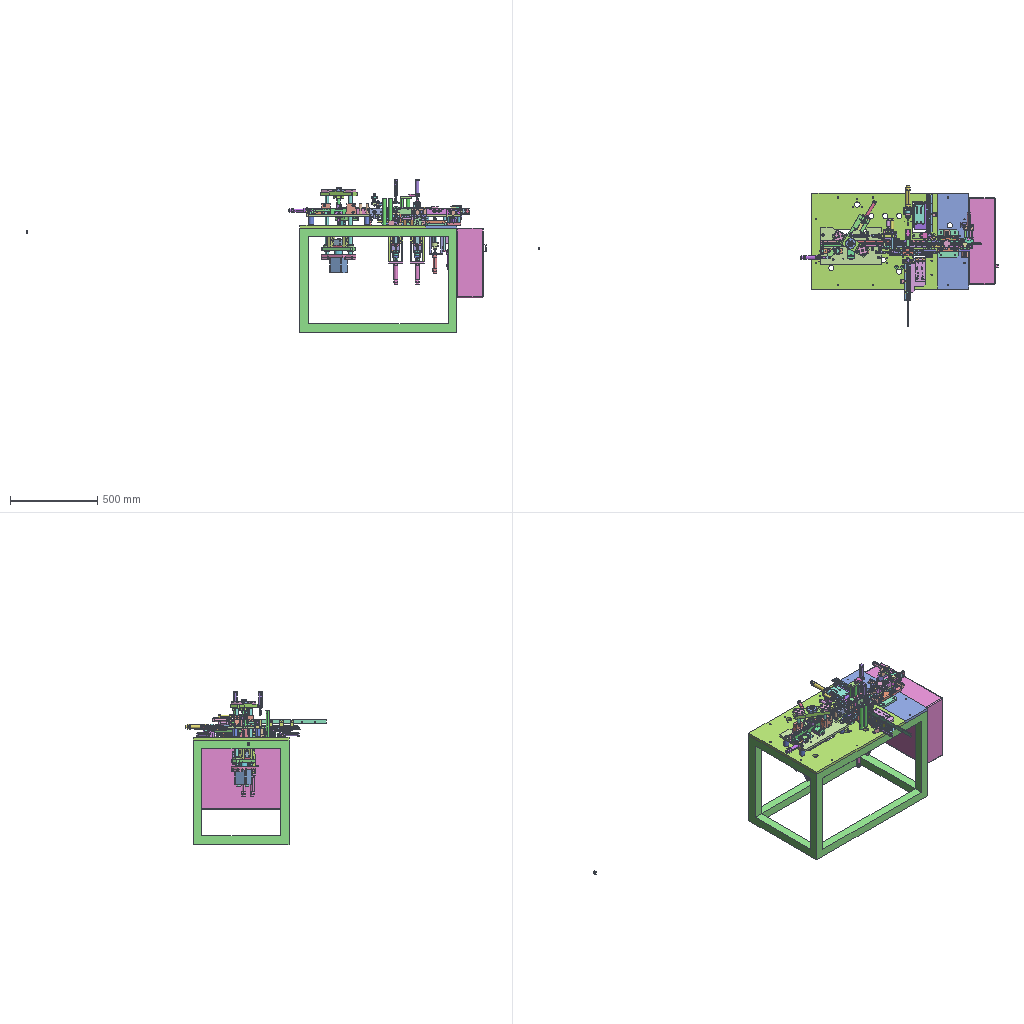Assembly | STEP file | 213 different items | 337 placed | box 2638 x 807 x 880 mm
Parts list (item | name | quantity | parent item | size | volume):
1 | magnet | x2 | in 180 magnet feeder main assembly | 5.5 x 14 x 19.5 mm | 770.904 mm3
2 | base plate | x1 | in 180 magnet feeder main assembly | 900 x 550 x 16 mm | 6619643 mm3
3 | vibratory feeder base plate | x2 | in vibratory feeder assembly | 116.996 x 12 x 60 mm | 79045 mm3
4 | vibratory feeder upper plate | x2 | in vibratory feeder assembly | 116.996 x 12 x 60 mm | 77221 mm3
5 | vibratory feeder support plate | x4 | in vibratory feeder assembly | 65 x 1 x 55 mm | 2512 mm3
6 | vibratory feeder support plate | x2 | in vibratory feeder assembly | 110 x 150 x 8 mm | 126115 mm3
7 | frame | x1 | in 180 magnet feeder main assembly | 550 x 600 x 900 mm | 18125000 mm3
8 | shell block | x3 | in 180 magnet feeder main assembly, 180 cup machine | 307.5 x 15.4 x 34 mm | 6550 mm3
9 | support plate 11 | x4 | in magnet input slingshot assembly | 8 x 160 x 68 mm | 53075 mm3
10 | slingshot push rod cylinder seat | x2 | in magnet input slingshot assembly | 81 x 35 x 8 mm | 19658 mm3
11 | CDM2B20-50-XC8 | x2 | in magnet input slingshot assembly | 24 x 24 x 166 mm | 54436 mm3
12 | magnetic tile top shaft cylinder seat 2 | x2 | in magnet input slingshot assembly | 45 x 49 x 12 mm | 14964 mm3
13 | top shaft cylinder seat support plate 2 | x2 | in magnet input slingshot assembly | 45 x 65 x 16 mm | 36671 mm3
14 | magnetic tile top shaft slide seat | x2 | in magnet input slingshot assembly | 95 x 90 x 26 mm | 105605 mm3
15 | union seat 11 | x2 | in magnet input slingshot assembly | 40 x 20 x 11 mm | 4585 mm3
16 | magnetic tile top shaft slider | x2 | in magnet input slingshot assembly | 40 x 51 x 45 mm | 61253 mm3
17 | slide seat cover plate 4 | x4 | in magnet input slingshot assembly | 17 x 90 x 10 mm | 13210 mm3
18 | union | x2 | in magnet input slingshot assembly | 16 x 17 x 16 mm | 2228 mm3
19 | magnetic tile top shaft | x2 | in magnet input slingshot assembly | 19 x 14 x 158 mm | 23396 mm3
20 | top shaft | x2 | in magnet input slingshot assembly | 8 x 11.5 x 178 mm | 13034 mm3
21 | union 1 | x2 | in magnet input slingshot assembly | 34 x 30 x 15 mm | 9782 mm3
22 | M6 screw | x2 | in magnet input slingshot assembly | 21 x 11 x 11 mm | 825.269 mm3
23 | CDM2B20-75 | x2 | in magnet input slingshot assembly | 24 x 24 x 166 mm | 54436 mm3
24 | push rod union | x2 | in magnet input slingshot assembly | 22 x 25 x 25 mm | 8188 mm3
25 | guide pin seat | x1 | in push slingshot assembly | 65 x 71 x 15 mm | 41839 mm3
26 | CDJ2B16_45_B_0_ | x5 | in push slingshot assembly, secondary slingshot input assembly, push material assembly | 18 x 22.7 x 120 mm | 25727 mm3
27 | slingshot displacement cylinder seat post | x4 | in push slingshot assembly, secondary slingshot input assembly | 20 x 20 x 155 mm | 47945 mm3
28 | push slingshot cylinder seat 2 | x2 | in push slingshot assembly, secondary slingshot input assembly | 60 x 26 x 20 mm | 12397 mm3
29 | slingshot track | x2 | in push slingshot assembly, secondary slingshot input assembly | 34 x 23.53 x 224 mm | 76613 mm3
30 | slingshot track fixed block | x3 | in push slingshot assembly | 11 x 40 x 22 mm | 2404 mm3
31 | secondary slingshot input track spacer block | x1 | in push slingshot assembly | 180 x 112 x 15 mm | 210119 mm3
32 | slingshot press plate | x1 | in push slingshot assembly | 375 x 20 x 5 mm | 36809 mm3
33 | pin seat 2 | x2 | in push slingshot assembly 9 | 35 x 30 x 8 mm | 7349 mm3
34 | pin seat 1 | x2 | in push slingshot assembly 9 | 35 x 30 x 8 mm | 7351 mm3
35 | slingshot push rod | x2 | in push slingshot assembly 9 | 16.072 x 21.6 x 67.5 mm | 5779 mm3
36 | union 4 | x2 | in push slingshot assembly, secondary slingshot input assembly | 12 x 21 x 12 mm | 1814 mm3
37 | lifting link plate | x2 | in push slingshot assembly, secondary slingshot input assembly | 13 x 40 x 8.5 mm | 2401 mm3
38 | fiber optic seat 2 | x2 | in push slingshot assembly, secondary slingshot input assembly | 13 x 13 x 13 mm | 515.025 mm3
39 | 16 union cap | x2 | in push slingshot assembly, secondary slingshot input assembly | 16 x 18 x 16 mm | 2782 mm3
40 | 16 union | x2 | in push slingshot assembly, secondary slingshot input assembly | 16 x 16 x 30 mm | 1888 mm3
41 | detection slide rod | x1 | in detection assembly | 60 x 12.5 x 13 mm | 5988 mm3
42 | detection union | x1 | in detection assembly | 19 x 12 x 14 mm | 1541 mm3
43 | slide seat | x2 | in detection assembly | 26 x 38 x 10 mm | 4433 mm3
44 | detection pin | x1 | in detection assembly | 6 x 6 x 30 mm | 164.036 mm3
45 | switch seat | x1 | in detection assembly | 35 x 29 x 12 mm | 1653 mm3
46 | detection post | x2 | in detection assembly | 16 x 16 x 60 mm | 11399 mm3
47 | push magnet block | x2 | in magnet input tile assembly | 25 x 14 x 20 mm | 5584 mm3
48 | push magnet union | x2 | in magnet input tile assembly | 10 x 10 x 18 mm | 1240 mm3
49 | push magnet block pin | x2 | in magnet input tile assembly | 3 x 3 x 14 mm | 98.96 mm3
50 | push magnet slide seat | x2 | in magnet input tile assembly | 34 x 28 x 32 mm | 18978 mm3
51 | push magnet slide seat spacer block | x2 | in magnet input tile assembly | 34 x 75 x 10 mm | 22964 mm3
52 | push magnet cylinder seat | x2 | in magnet input tile assembly | 34 x 25 x 28 mm | 8909 mm3
53 | push magnet seat spacer block 1 | x2 | in magnet input tile assembly | 34 x 20 x 17 mm | 10432 mm3
54 | magnet input block | x1 | in magnet input tile assembly | 60 x 40 x 64 mm | 101376 mm3
55 | CDJ2B10_30_C76_0_ | x2 | in magnet input tile assembly | 12.2 x 35.4 x 104 mm | 14245 mm3
56 | secondary slingshot input support plate | x1 | in secondary slingshot input assembly | 30 x 12 x 65 mm | 21465 mm3
57 | slingshot displacement cylinder seat | x1 | in secondary slingshot input assembly | 30 x 60 x 10 mm | 13257 mm3
58 | slider | x1 | in secondary slingshot input assembly | 80 x 40 x 8.5 mm | 14605 mm3
59 | slide seat 2 | x1 | in secondary slingshot input assembly | 65 x 30 x 80 mm | 57005 mm3
60 | secondary slingshot input track spacer block 1 | x1 | in secondary slingshot input assembly | 150 x 100 x 15 mm | 181436 mm3
61 | secondary slingshot input seat | x1 | in track assembly | 52 x 40 x 50 mm | 79247 mm3
62 | track spacer block 1 | x1 | in track assembly | 60 x 50 x 15 mm | 33797 mm3
63 | track spacer block 2 | x1 | in track assembly | 60 x 50 x 15 mm | 33477 mm3
64 | magnetizing track | x1 | in track assembly | 40 x 14 x 120 mm | 55579 mm3
65 | magnetizing side block 2 | x1 | in track assembly | 120 x 12.3 x 34.5 mm | 45166 mm3
66 | magnetizing side block | x1 | in track assembly | 120 x 12.3 x 34.5 mm | 44752 mm3
67 | secondary slingshot input side block 1 | x1 | in track assembly | 82.5 x 12.3 x 34.5 mm | 28839 mm3
68 | secondary slingshot input track | x1 | in track assembly | 40 x 14 x 82.5 mm | 35227 mm3
69 | iron shell displacement union | x1 | in track assembly | 15 x 22 x 39 mm | 5236 mm3
70 | iron shell displacement union seat | x1 | in track assembly | 27 x 25 x 18 mm | 8727 mm3
71 | track support post | x2 | in track assembly | 15 x 15 x 24 mm | 3445 mm3
72 | CDM2B20-50 | x1 | in track assembly | 24 x 24 x 166 mm | 54436 mm3
73 | insert limit | x8 | in track assembly, 180 magnet feeder main assembly | 20 x 12 x 10 mm | 1551 mm3
74 | iron shell positioning insert | x8 | in track assembly, 180 magnet feeder main assembly | 24 x 16.5 x 5 mm | 1571 mm3
75 | side block 5 | x1 | in track assembly | 12.1 x 101.5 x 34.5 mm | 29782 mm3
76 | side block 4 | x1 | in track assembly | 12.1 x 101.5 x 34.5 mm | 36196 mm3
77 | track (2) | x1 | in track assembly | 101.5 x 40 x 14 mm | 49700 mm3
78 | displacement block | x1 | in track assembly | 26.6 x 105 x 40.2 mm | 48167 mm3
79 | track (3) | x1 | in track assembly | 140 x 40 x 16 mm | 70636 mm3
80 | side block 3-2 | x1 | in track assembly | 39.2 x 12.1 x 34.5 mm | 13891 mm3
81 | side block 3 | x1 | in track assembly | 39.196 x 12.1 x 34.5 mm | 14030 mm3
82 | side block 2-2 | x1 | in track assembly | 80.6 x 12.1 x 34.5 mm | 30402 mm3
83 | side block 2 | x1 | in track assembly | 80.434 x 12.1 x 34.5 mm | 30816 mm3
84 | spacer block 4 | x1 | in track assembly | 115 x 40 x 48 mm | 178112 mm3
85 | cylinder seat 2 | x1 | in track assembly | 52 x 38.5 x 25 mm | 17688 mm3
86 | spacer block 5 | x1 | in track assembly | 52 x 30 x 37 mm | 53755 mm3
87 | cylinder positioning fork | x3 | in track assembly | 20 x 21.799 x 12 mm | 3903 mm3
88 | CDQ2B16-5D | x3 | in track assembly | 29.349 x 29.349 x 39 mm | 26194 mm3
89 | positioning cylinder plate | x2 | in track assembly | 70 x 20 x 8 mm | 10113 mm3
90 | positioning cylinder post | x6 | in track assembly | 10 x 10 x 15 mm | 821.723 mm3
91 | magnetizing cover plate | x1 | in track assembly | 40 x 10 x 40 mm | 14400 mm3
92 | POM limit 1 | x1 | in track assembly | 30 x 30 x 19 mm | 11486 mm3
93 | cover plate | x1 | in track assembly | 66.95 x 15 x 6 mm | 5439 mm3
94 | cover plate 2 | x1 | in track assembly | 97 x 15 x 6 mm | 8008 mm3
95 | cover plate 3 | x1 | in track assembly | 20.5 x 55 x 10 mm | 9961 mm3
96 | cover plate 4 | x1 | in track assembly | 155 x 6 x 12 mm | 10035 mm3
97 | cover plate 5 | x1 | in track assembly | 60 x 15 x 6 mm | 4845 mm3
98 | detection track | x1 | in track assembly | 40 x 14 x 80 mm | 36343 mm3
99 | detection side block left | x1 | in track assembly | 80 x 12.3 x 34.5 mm | 25865 mm3
100 | detection side block right | x1 | in track assembly | 45 x 12.3 x 28 mm | 12527 mm3
101 | iron shell positioning insert-1 | x1 | in track assembly | 20 x 16.011 x 5 mm | 1177 mm3
102 | positioning cylinder plate-1 | x1 | in track assembly | 50 x 25 x 8 mm | 9039 mm3
103 | limit pin-1 | x1 | in track assembly | 12 x 18.5 x 8 mm | 1103 mm3
104 | limit block-1 | x1 | in track assembly | 16 x 9 x 10 mm | 904.118 mm3
105 | track post-1 | x2 | in track assembly | 15 x 15 x 35 mm | 5353 mm3
106 | detection track cover plate | x1 | in track assembly | 30 x 27 x 10 mm | 6611 mm3
107 | BU-C06-2 | x1 | in 180 cup machine | 40 x 60 x 14 mm | 23429 mm3
108 | BU-C06-1 | x1 | in 180 cup machine | 40 x 60 x 10 mm | 21287 mm3
109 | BU-C08b-2 | x1 | in 180 cup machine | 5 x 30 x 5 mm | 576.997 mm3
110 | BU-C08b-1 | x2 | in 180 cup machine, 180 cup material feed assembly | 5 x 22 x 5 mm | 419.918 mm3
111 | BU-A12 | x1 | in assembly 3 | 216 x 25 x 60 mm | 252234 mm3
112 | BU-A01-2 | x4 | in assembly 3, 180 cup machine | 49 x 50 x 14 mm | 28416 mm3
113 | BU-A02a | x2 | in assembly 3 | 375 x 20 x 20 mm | 113660 mm3
114 | BU-E02 | x1 | in assembly 4 | 20 x 26 x 17 mm | 2778 mm3
115 | BU-A05 | x1 | in assembly 4 | 206 x 50 x 20 mm | 148133 mm3
116 | BU-A04 | x1 | in assembly 4 | 206 x 50 x 20 mm | 161458 mm3
117 | BU-A20 | x1 | in assembly 4 | 30 x 60 x 50 mm | 38782 mm3
118 | CDQ2B32-10-A73 | x1 | in assembly 4 | 44.99 x 40 x 44.982 mm | 63998 mm3
119 | BU-A03a | x2 | in assembly 4 | 50 x 80 x 18 mm | 61790 mm3
120 | BU-A06#180 | x1 | in assembly 6- cup | 48 x 68.5 x 48 mm | 23546 mm3
121 | BU-A07#180 | x1 | in assembly 6- cup | 26 x 63 x 26 mm | 8732 mm3
122 | BU-A08 | x1 | in assembly 6- cup | 4.5 x 27 x 4.5 mm | 144.202 mm3
123 | BU-A09 | x1 | in assembly 6- cup | 38.05 x 4.5 x 4.5 mm | 179.303 mm3
124 | BU-A15a | x4 | in assembly 4 | 40 x 40 x 7.5 mm | 3393 mm3
125 | BU-A01 | x1 | in 180 cup machine | 205 x 75 x 15 mm | 173838 mm3
126 | BU-A02b | x1 | in 180 cup machine | 45 x 45 x 25 mm | 31907 mm3
127 | BU-A13#130b | x1 | in assembly 2 | 22 x 7 x 7 mm | 944.521 mm3
128 | BU-E01#130 | x1 | in assembly 2 | 30 x 30 x 23 mm | 11677 mm3
129 | BU-A13#130a | x1 | in assembly 2 | 30 x 110 x 30 mm | 44972 mm3
130 | BU-A19-1 | x1 | in assembly 2 | 28 x 28 x 3 mm | 1635 mm3
131 | BU-A14a | x1 | in 180 cup machine | 60 x 12 x 60 mm | 23804 mm3
132 | BU-A14b | x1 | in 180 cup machine | 60 x 13.5 x 60 mm | 27218 mm3
133 | BU-B02 | x1 | in assembly 5 | 62 x 12 x 9 mm | 4933 mm3
134 | BU-B05b | x1 | in assembly 5 | 50 x 25 x 5 mm | 5231 mm3
135 | BU-B05a | x1 | in assembly 5 | 56 x 40 x 8 mm | 14978 mm3
136 | BU-B05c | x1 | in assembly 5 | 14 x 15 x 12 mm | 1515 mm3
137 | BU-B01 | x1 | in assembly 5 | 143 x 68 x 22 mm | 122394 mm3
138 | 5 | x2 | in A_CDJ2B16-60-B | 18 x 18 x 115 mm | 25719 mm3
139 | 6 | x2 | in A_CDJ2B16-60-B | 5 x 5 x 81 mm | 1576 mm3
140 | BU-B04 | x1 | in assembly 8 | 105 x 20 x 9 mm | 16085 mm3
141 | BU-B03#260 | x1 | in assembly 8 | 37 x 19.6 x 4 mm | 1912 mm3
142 | BU-A11 | x2 | in assembly 7 | 65 x 60 x 30 mm | 72438 mm3
143 | BU-A15b | x4 | in assembly 7 | 13 x 11.5 x 13 mm | 1411 mm3
144 | BU-A15c | x4 | in assembly 7 | 13 x 11.5 x 13 mm | 1326 mm3
145 | BU-D02#180c | x2 | in 180 cup machine | 115 x 32.5 x 9 mm | 31043 mm3
146 | 3 | x1 | in CDQ2B12-5D | 25.087 x 25.087 x 33 mm | 16395 mm3
147 | 4 | x1 | in CDQ2B12-5D | 6 x 6 x 15.5 mm | 398.486 mm3
148 | BU-C07#180 | x1 | in 180 cup machine | 32 x 86.655 x 8 mm | 11719 mm3
149 | BU-D02#180a | x1 | in 180 cup machine | 235 x 32.5 x 9 mm | 55539 mm3
150 | BU-D02#180b | x1 | in 180 cup machine | 235 x 32.5 x 9 mm | 66956 mm3
151 | CDQ2B63-50D-A73 | x1 | in 180 cup machine | 77 x 94 x 77.01 mm | 486340 mm3
152 | BU-D02-2a#180 | x1 | in 180 cup machine | 177 x 17 x 7 mm | 20122 mm3
153 | BU-D02-2b#180 | x1 | in 180 cup machine | 173.003 x 17 x 7 mm | 19694 mm3
154 | BU-C02 | x2 | in 180 cup material feed assembly | 45 x 24 x 16 mm | 10831 mm3
155 | BU-C01 | x1 | in 180 cup material feed assembly | 126 x 18 x 28 mm | 33069 mm3
156 | BU-C04 | x1 | in 180 cup material feed assembly | 66 x 10 x 10 mm | 4793 mm3
157 | BU-C03a | x1 | in 180 cup material feed assembly | 40 x 52 x 6 mm | 8821 mm3
158 | BU-C03b | x1 | in 180 cup material feed assembly | 14 x 19 x 14 mm | 1370 mm3
159 | BU-C05-1 | x1 | in 180 cup material feed assembly | 16 x 28 x 16 mm | 4723 mm3
160 | cup material feed cylinder seat | x1 | in 180 cup material feed assembly | 12 x 50 x 40 mm | 15090 mm3
161 | CDM2B20-25 | x2 | in 180 cup material feed assembly, magnet, slingshot detection machine mechanism | 24 x 24 x 141 mm | 45275 mm3
162 | M6 | x2 | in 180 cup material feed assembly | 10 x 29.55 x 10 mm | 1049 mm3
163 | bore 20 linear bearing | x4 | in 180 cup machine | 32 x 32 x 42 mm | 19566 mm3
164 | BU-A03b#180 | x4 | in 180 cup machine | 29 x 29 x 51 mm | 31619 mm3
165 | middle plate | x2 | in 180 cup machine | 350 x 210 x 13 mm | 812608 mm3
166 | electrical control box | x1 | in 180 magnet feeder main assembly | 500 x 400 x 167 mm | 29965916 mm3
167 | slideway | x1 | in push material assembly | 80 x 30 x 12 mm | 20799 mm3
168 | slider 2 | x1 | in push material assembly | 19.196 x 10 x 120 mm | 18133 mm3
169 | positioning fork | x1 | in push material assembly | 40.8 x 43.762 x 8 mm | 6960 mm3
170 | slideway cylinder seat | x1 | in push material assembly | 12 x 35 x 50 mm | 15461 mm3
171 | slider cylinder plate | x1 | in push material assembly | 50 x 20 x 23.5 mm | 9756 mm3
172 | JA15_5_080 | x1 | in push material assembly | 16 x 16 x 34.5 mm | 3402 mm3
173 | push seat | x1 | in push material assembly | 75 x 15 x 20 mm | 19572 mm3
174 | CDJ2B16-15-B | x1 | in push material assembly | 18 x 18 x 90 mm | 16817 mm3
175 | magnetizing base plate | x1 | in magnetizing assembly | 160 x 120 x 12 mm | 139548 mm3
176 | bearing pad plate | x1 | in magnetizing assembly | 90 x 120 x 14 mm | 116838 mm3
177 | magnetizing cylinder plate post | x4 | in magnetizing assembly | 12 x 12 x 174 mm | 19275 mm3
178 | rotary cylinder plate | x1 | in magnetizing assembly | 125 x 80 x 8 mm | 54016 mm3
179 | magnetizing head 3 | x1 | in magnetizing | 13 x 11.779 x 35 mm | 1900 mm3
180 | magnetizing head 2 | x1 | in magnetizing | 23.5 x 24 x 120 mm | 49065 mm3
181 | magnetizing head 1 | x1 | in magnetizing | 19 x 14 x 38 mm | 5895 mm3
182 | magnetizing head 2-2 | x1 | in magnetizing | 19 x 14 x 62 mm | 8649 mm3
183 | union washer | x1 | in magnetizing assembly | 30 x 25 x 11 mm | 6415 mm3
184 | CDM2B20-35 | x1 | in magnetizing assembly | 24 x 24 x 151 mm | 48940 mm3
185 | magnetizing guide plate | x1 | in magnetizing assembly | 80 x 60 x 12 mm | 43374 mm3
186 | union head A | x1 | in magnetizing assembly | 40 x 36 x 40 mm | 19001 mm3
187 | turning shaft | x1 | in turning assembly | 20 x 18 x 45.6 mm | 3898 mm3
188 | deep groove bearing 6800 | x2 | in turning assembly | 19 x 19 x 5 mm | 1002 mm3
189 | spur gear_iso_ISO - Spur gear 1M 17T 20PA 10FW ---S17A75H50L0.8N | x1 | in turning assembly | 10 x 18.879 x 18.957 mm | 2165 mm3
190 | turning cylinder seat | x1 | in turning assembly | 38 x 85 x 21 mm | 18885 mm3
191 | locking washer | x1 | in turning assembly | 15 x 15 x 3 mm | 458.869 mm3
192 | hexagon socket head cap screws gb_GB_FASTENER_SCREWS_HSHCS M5X8-N | x1 | in turning assembly | 13 x 8.5 x 8.5 mm | 398.856 mm3
193 | rack spur rectangular_iso_ISO - Rack-spur - rectangular 1M 20PA 10FW 12PH 60L---SAll | x1 | in turning assembly | 60 x 13 x 10 mm | 7063 mm3
194 | CDJ2B16-30-B | x1 | in turning assembly | 18 x 22.7 x 105 mm | 21828 mm3
195 | detection slide seat--1 | x1 | in magnet, slingshot detection machine mechanism | 105 x 90 x 27 mm | 120388 mm3
196 | detection slider--1 | x1 | in magnet, slingshot detection machine mechanism | 48 x 52 x 45 mm | 66698 mm3
197 | detection union--1 | x1 | in magnet, slingshot detection machine mechanism | 16 x 17 x 16 mm | 2228 mm3
198 | detection union seat--1 | x1 | in magnet, slingshot detection machine mechanism | 40 x 20 x 11 mm | 4585 mm3
199 | detection slide seat cover plate--1 | x2 | in magnet, slingshot detection machine mechanism | 17.5 x 90 x 7 mm | 9559 mm3
200 | detection cylinder seat--1 | x1 | in magnet, slingshot detection machine mechanism | 45 x 45 x 12 mm | 14666 mm3
201 | detection cylinder seat support plate--1 | x1 | in magnet, slingshot detection machine mechanism | 45 x 75 x 12 mm | 34324 mm3
202 | slingshot detection spring block | x2 | in magnet, slingshot detection machine mechanism | 4.5 x 7.6 x 97 mm | 2316 mm3
203 | magnetic tile slingshot detection base seat | x1 | in magnet, slingshot detection machine mechanism | 25 x 27 x 163 mm | 57664 mm3
204 | magnetic tile detection pin | x2 | in magnet, slingshot detection machine mechanism | 6 x 99 x 6 mm | 816.507 mm3
205 | slingshot detection positioning | x1 | in magnet, slingshot detection machine mechanism | 60 x 80 x 15 mm | 59930 mm3
206 | spring | x2 | in magnet, slingshot detection machine mechanism | 5.998 x 5.998 x 20.499 mm | 67.793 mm3
207 | spring-1 | x2 | in magnet, slingshot detection machine mechanism | 3.998 x 3.998 x 20.249 mm | 43.124 mm3
208 | discharge block | x1 | in defective part material split assembly | 48.4 x 33 x 52 mm | 23054 mm3
209 | defective part push material cylinder seat | x1 | in defective part material split assembly | 30 x 45 x 60 mm | 39635 mm3
210 | material split support plate | x1 | in defective part material split assembly | 27 x 66 x 75 mm | 51635 mm3
211 | slide rod | x2 | in defective part material split assembly | 8 x 8 x 87 mm | 4373 mm3
212 | CDJ2B16_30-B | x1 | in defective part material split assembly | 18 x 22.7 x 120 mm | 25727 mm3
213 | linear bearing LM8-8-15-24 | x2 | in defective part material split assembly | 24 x 15 x 15 mm | 2989 mm3
Placements (level | parent | child | x y z in mm | rotation matrix by rows), first 333 of 367 lines:
1 | 180 magnet feeder main assembly | magnet | 1608.938 -339.0 35.755 | 1 0 0 0 1 0 0 0 1
1 | 180 magnet feeder main assembly | magnet | 1608.938 -339.0 1.44 | -1 0 0 0 1 0 0 0 -1
1 | 180 magnet feeder main assembly | base plate | 1608.938 -330.0 -16.0 | 1 0 0 0 1 0 0 0 1
1 | 180 magnet feeder main assembly | vibratory feeder assembly | 1703.938 -147.447 -13.05 | 0 0 -1 -1 0 0 0 1 -0
2 | vibratory feeder assembly | vibratory feeder base plate | -66.165 -2.95 -0.0 | 1 0 0 0 1 0 0 0 1
2 | vibratory feeder assembly | vibratory feeder upper plate | 32.453 59.542 -0.0 | -1 0 0 0 -1 0 0 0 1
2 | vibratory feeder assembly | vibratory feeder support plate | -85.529 59.328 57.5 | 0.342 0.9397 0 -0.9397 0.342 0 0 0 1
2 | vibratory feeder assembly | vibratory feeder support plate | 28.04 59.666 57.5 | 0.342 0.9397 0 -0.9397 0.342 0 0 0 1
2 | vibratory feeder assembly | vibratory feeder support plate | -12.844 -2.95 67.832 | -1 0 0 0 0 -1 0 -1 -0
1 | 180 magnet feeder main assembly | frame | 1958.938 -80.97 -80.128 | 0 0 -1 1 0 0 0 -1 -0
1 | 180 magnet feeder main assembly | shell block | 1731.938 -289.8 64.0 | 1 0 0 0 1 0 0 0 1
1 | 180 magnet feeder main assembly | magnet input slingshot assembly | 1572.997 -332.019 -229.271 | 1 0 0 0 0 1 0 -1 0
2 | magnet input slingshot assembly | support plate 11 | 46.899 -101.093 -26.981 | 1 0 0 0 1 0 0 0 1
2 | magnet input slingshot assembly | support plate 11 | -26.101 -101.093 -26.981 | 1 0 0 0 1 0 0 0 1
2 | magnet input slingshot assembly | slingshot push rod cylinder seat | 35.841 -12.971 -6.981 | 1 0 0 0 0 -1 0 1 0
2 | magnet input slingshot assembly | CDM2B20-50-XC8 | 35.941 -86.026 23.019 | 1 0 0 0 0 -1 0 1 0
2 | magnet input slingshot assembly | magnetic tile top shaft cylinder seat 2 | 35.941 -73.026 23.019 | -1 0 0 0 0 -1 0 -1 0
2 | magnet input slingshot assembly | top shaft cylinder seat support plate 2 | 46.476 -155.631 41.019 | 1 0 0 0 1 0 0 0 1
2 | magnet input slingshot assembly | magnetic tile top shaft slide seat | -0.6732 -207.695 41.019 | -1 0 0 0 1 0 0 0 -1
2 | magnet input slingshot assembly | union seat 11 | 73.591 -112.026 12.598 | -1 0 0 0 0 -1 0 -1 -0
2 | magnet input slingshot assembly | magnetic tile top shaft slider | 35.941 -123.026 -6.981 | -1 0 0 0 0 -1 0 -1 0
2 | magnet input slingshot assembly | slide seat cover plate 4 | 58.192 -176.171 17.019 | 1 0 0 0 -1 0 0 0 -1
2 | magnet input slingshot assembly | slide seat cover plate 4 | 13.489 -160.37 17.019 | -1 0 0 0 1 0 0 0 -1
2 | magnet input slingshot assembly | union | 35.941 -114.526 23.019 | 0.9287 0 0.3708 0 1 0 -0.3708 0 0.9287
2 | magnet input slingshot assembly | magnetic tile top shaft | 35.941 -281.026 -6.981 | -1 0 0 0 0 1 0 1 0
2 | magnet input slingshot assembly | top shaft | 35.941 -14.626 -6.981 | 1 0 0 0 0 -1 0 1 0
2 | magnet input slingshot assembly | union 1 | 18.941 -74.626 -14.481 | 1 0 0 0 1 0 0 0 1
2 | magnet input slingshot assembly | M6 screw | 32.194 -71.797 -3.095 | 0 -0.6941 -0.7198 -1 0 0 0 0.7198 -0.6941
2 | magnet input slingshot assembly | CDM2B20-75 | 35.841 -25.971 -6.981 | 1 0 0 0 0 -1 0 1 0
2 | magnet input slingshot assembly | push rod union | 35.941 -66.648 -6.981 | 1 0 0 0 1 0 0 0 1
1 | 180 magnet feeder main assembly | push slingshot assembly | 1658.677 -395.625 44.596 | 1 0 0 0 1 0 0 0 1
2 | push slingshot assembly | guide pin seat | -79.888 6.625 22.123 | 1 0 0 0 0 -1 0 1 0
2 | push slingshot assembly | CDJ2B16_45_B_0_ | -49.742 10.225 119.404 | -0.9237 -0.383 0 -0.383 0.9237 0 0 0 -1
2 | push slingshot assembly | slingshot displacement cylinder seat post | -79.742 -30.275 -44.596 | 1 0 0 0 1 0 0 0 1
2 | push slingshot assembly | slingshot displacement cylinder seat post | -114.742 -30.275 -44.596 | 1 0 0 0 1 0 0 0 1
2 | push slingshot assembly | push slingshot cylinder seat 2 | -59.545 -101.775 6.577 | 1 0 0 0 0 -1 0 1 -0
2 | push slingshot assembly | CDJ2B16_45_B_0_ | -49.74 -113.775 -29.596 | 1 0 0 0 0 1 0 -1 0
2 | push slingshot assembly | slingshot track | -48.712 2.822 18.073 | 1 0 0 0 0 -1 0 1 -0
2 | push slingshot assembly | slingshot track fixed block | -70.239 -40.178 12.674 | 1 0 0 0 0 -1 0 1 0
2 | push slingshot assembly | secondary slingshot input track spacer block | 11.663 -74.429 -12.326 | 0 1 0 -1 0 0 0 0 1
2 | push slingshot assembly | slingshot press plate | -52.248 6.322 35.673 | 0 0 1 -1 0 0 0 -1 0
2 | push slingshot assembly | slingshot track fixed block | -70.239 -100.178 12.674 | 1 0 0 0 0 -1 0 1 -0
2 | push slingshot assembly | slingshot track fixed block | -70.239 -160.178 12.674 | 1 0 0 0 0 -1 0 1 0
2 | push slingshot assembly | push slingshot assembly 9 | -49.654 -62.272 -31.141 | 1 0 0 0 0 -1 0 1 0
3 | push slingshot assembly 9 | pin seat 2 | -0.086 -13.455 1.11 | 1 0 0 0 1 0 0 0 1
3 | push slingshot assembly 9 | pin seat 1 | -0.086 -13.455 9.11 | 1 0 0 0 1 0 0 0 1
3 | push slingshot assembly 9 | slingshot push rod | -0.086 11.545 -58.39 | 1 0 0 0 1 0 0 0 1
2 | push slingshot assembly | union 4 | -49.742 10.225 85.404 | 0.9996 0 0.02919 0.02919 0 -0.9996 0 1 -0
2 | push slingshot assembly | lifting link plate | -49.74 6.875 80.404 | 0 1 0 0 0 1 1 0 -0
2 | push slingshot assembly | fiber optic seat 2 | -49.74 29.712 24.304 | 0 1 0 -1 0 0 0 0 1
2 | push slingshot assembly | 16 union cap | -48.096 -98.802 -32.645 | -0.4746 0 0.8802 0 -1 0 0.8802 0 0.4746
2 | push slingshot assembly | 16 union | -49.74 -101.285 -29.596 | -0.4634 0.8862 0 0 0 1 0.8862 0.4634 0
1 | 180 magnet feeder main assembly | shell block | 2018.938 -289.8 64.0 | 1 0 0 0 1 0 0 0 1
1 | 180 magnet feeder main assembly | detection assembly | 1467.491 -300.936 150.688 | 0 -0.01093 0.9999 0 0.9999 0.01093 -1 0 0
2 | detection assembly | detection slide rod | -25.062 7.104 19.0 | 1 0 0 0 0 -1 0 1 0
2 | detection assembly | detection union | -28.062 1.104 19.0 | 1 0 0 0 1 0 0 0 1
2 | detection assembly | slide seat | 21.938 7.104 19.0 | 0 0 1 0 1 0 -1 0 0
2 | detection assembly | slide seat | -15.062 7.104 19.0 | 0 0 1 0 1 0 -1 0 0
2 | detection assembly | detection pin | 44.938 7.104 19.0 | 0 0 -1 0.6521 -0.7581 0 -0.7581 -0.6521 -0
2 | detection assembly | switch seat | -3.055 -2.396 20.5 | 1 0 0 0 0 -1 0 1 -0
2 | detection assembly | detection post | 86.688 -17.896 -61.75 | 0 0 -1 0 1 0 1 0 0
2 | detection assembly | detection post | 86.688 -17.896 -21.75 | 0 0 -1 -0.8482 0.5297 0 0.5297 0.8482 0
1 | 180 magnet feeder main assembly | magnet input slingshot assembly | 1696.231 -283.019 -229.271 | 1 0 0 0 0 1 0 -1 -0
2 | magnet input slingshot assembly | support plate 11 | 46.899 -101.093 -26.981 | 1 0 0 0 1 0 0 0 1
2 | magnet input slingshot assembly | support plate 11 | -26.101 -101.093 -26.981 | 1 0 0 0 1 0 0 0 1
2 | magnet input slingshot assembly | slingshot push rod cylinder seat | 35.841 -12.971 -6.981 | 1 0 0 0 0 -1 0 1 0
2 | magnet input slingshot assembly | CDM2B20-50-XC8 | 35.941 -86.026 23.019 | 1 0 0 0 0 -1 0 1 0
2 | magnet input slingshot assembly | magnetic tile top shaft cylinder seat 2 | 35.941 -73.026 23.019 | -1 0 0 0 0 -1 0 -1 0
2 | magnet input slingshot assembly | top shaft cylinder seat support plate 2 | 46.476 -155.631 41.019 | 1 0 0 0 1 0 0 0 1
2 | magnet input slingshot assembly | magnetic tile top shaft slide seat | -0.6732 -207.695 41.019 | -1 0 0 0 1 0 0 0 -1
2 | magnet input slingshot assembly | union seat 11 | 73.591 -112.026 12.598 | -1 0 0 0 0 -1 0 -1 -0
2 | magnet input slingshot assembly | magnetic tile top shaft slider | 35.941 -123.026 -6.981 | -1 0 0 0 0 -1 0 -1 0
2 | magnet input slingshot assembly | slide seat cover plate 4 | 58.192 -176.171 17.019 | 1 0 0 0 -1 0 0 0 -1
2 | magnet input slingshot assembly | slide seat cover plate 4 | 13.489 -160.37 17.019 | -1 0 0 0 1 0 0 0 -1
2 | magnet input slingshot assembly | union | 35.941 -114.526 23.019 | 0.9287 0 0.3708 0 1 0 -0.3708 0 0.9287
2 | magnet input slingshot assembly | magnetic tile top shaft | 35.941 -281.026 -6.981 | -1 0 0 0 0 1 0 1 0
2 | magnet input slingshot assembly | top shaft | 35.941 -14.626 -6.981 | 1 0 0 0 0 -1 0 1 0
2 | magnet input slingshot assembly | union 1 | 18.941 -74.626 -14.481 | 1 0 0 0 1 0 0 0 1
2 | magnet input slingshot assembly | M6 screw | 32.194 -71.797 -3.095 | 0 -0.6941 -0.7198 -1 0 0 0 0.7198 -0.6941
2 | magnet input slingshot assembly | CDM2B20-75 | 35.841 -25.971 -6.981 | 1 0 0 0 0 -1 0 1 0
2 | magnet input slingshot assembly | push rod union | 35.941 -66.648 -6.981 | 1 0 0 0 1 0 0 0 1
1 | 180 magnet feeder main assembly | vibratory feeder assembly | 1650.757 -420.996 -13.05 | 0 0 1 1 0 0 0 1 0
2 | vibratory feeder assembly | vibratory feeder base plate | -66.165 -2.95 -0.0 | 1 0 0 0 1 0 0 0 1
2 | vibratory feeder assembly | vibratory feeder upper plate | 32.453 59.542 -0.0 | -1 0 0 0 -1 0 0 0 1
2 | vibratory feeder assembly | vibratory feeder support plate | -85.529 59.328 57.5 | 0.342 0.9397 0 -0.9397 0.342 0 0 0 1
2 | vibratory feeder assembly | vibratory feeder support plate | 28.04 59.666 57.5 | 0.342 0.9397 0 -0.9397 0.342 0 0 0 1
2 | vibratory feeder assembly | vibratory feeder support plate | -12.844 -2.95 67.832 | -1 0 0 0 0 -1 0 -1 -0
1 | 180 magnet feeder main assembly | magnet input tile assembly | 1725.944 -351.136 31.424 | 1 0 0 0 1 0 0 0 1
2 | magnet input tile assembly | push magnet block | -49.506 12.136 3.576 | 1 0 0 0 1 0 0 0 1
2 | magnet input tile assembly | push magnet union | -50.006 12.136 13.576 | 0 0 1 0 -1 0 1 0 0
2 | magnet input tile assembly | push magnet block pin | -45.006 5.136 13.576 | -0.291 0.9567 0 0 0 1 0.9567 0.291 -0
2 | magnet input tile assembly | push magnet slide seat | -87.006 12.136 9.576 | 0 0 1 1 0 0 0 1 0
2 | magnet input tile assembly | push magnet slide seat spacer block | -71.006 12.136 -14.424 | 0 -1 0 1 0 0 0 0 1
2 | magnet input tile assembly | push magnet cylinder seat | -12.006 12.136 13.576 | 0 -1 0 -1 0 0 0 0 -1
2 | magnet input tile assembly | push magnet seat spacer block 1 | -47.006 12.136 -31.424 | 0 -1 0 1 0 0 0 0 1
2 | magnet input tile assembly | magnet input block | -117.006 -12.864 -31.424 | 1 0 0 0 1 0 0 0 1
2 | magnet input tile assembly | push magnet slide seat | -147.006 12.136 9.576 | 0 0 -1 -1 0 0 0 1 -0
2 | magnet input tile assembly | push magnet slide seat spacer block | -163.006 12.136 -14.424 | 0 1 0 -1 0 0 0 0 1
2 | magnet input tile assembly | push magnet seat spacer block 1 | -187.006 12.136 -31.424 | 0 -1 0 1 0 0 0 0 1
2 | magnet input tile assembly | push magnet cylinder seat | -222.006 12.136 13.576 | 0 1 0 1 0 0 0 0 -1
2 | magnet input tile assembly | push magnet block | -184.509 12.136 23.576 | -1 0 0 0 1 0 0 0 -1
2 | magnet input tile assembly | push magnet union | -184.009 12.136 13.576 | 0 0 -1 0 1 0 1 0 -0
2 | magnet input tile assembly | push magnet block pin | -189.009 5.136 13.576 | -0.291 0.9567 0 0 0 1 0.9567 0.291 -0
2 | magnet input tile assembly | CDJ2B10_30_C76_0_ | -214.006 12.136 13.576 | 0 0 1 1 0 0 0 1 0
2 | magnet input tile assembly | CDJ2B10_30_C76_0_ | -20.006 12.136 13.576 | 0 0 -1 -1 0 0 0 1 -0
1 | 180 magnet feeder main assembly | secondary slingshot input assembly | 1703.794 -241.773 160.158 | 0 0 -1 -1 0 0 0 1 0
2 | secondary slingshot input assembly | secondary slingshot input support plate | 1.727 0.8423 5.129 | 1 0 0 0 1 0 0 0 1
2 | secondary slingshot input assembly | slingshot displacement cylinder seat | 15.876 6.842 9.506 | 1 0 0 0 0 1 0 -1 0
2 | secondary slingshot input assembly | CDJ2B16_45_B_0_ | 1.727 3.842 -28.371 | -0.4064 0.9137 0 0 0 -1 -0.9137 -0.4064 -0
2 | secondary slingshot input assembly | slingshot displacement cylinder seat post | 1.727 -160.158 25.129 | 0 1 0 0 0 1 1 0 0
2 | secondary slingshot input assembly | slingshot displacement cylinder seat post | 1.727 -160.158 60.129 | -0.9634 -0.2681 0 0 0 1 -0.2681 0.9634 0
2 | secondary slingshot input assembly | slider | 6.727 -60.158 -11.927 | 0 0 -1 1 0 0 0 -1 0
2 | secondary slingshot input assembly | slide seat 2 | -8.398 -160.158 21.362 | 0 1 0 0 0 1 1 0 0
2 | secondary slingshot input assembly | push slingshot cylinder seat 2 | -110.273 -108.975 -38.182 | 0 0 -1 0 1 0 1 0 0
2 | secondary slingshot input assembly | CDJ2B16_45_B_0_ | -122.273 -145.148 -28.377 | 0 0 1 0 -1 0 1 0 -0
2 | secondary slingshot input assembly | slingshot track | -7.575 -100.388 -27.35 | 0 0 -1 0 1 0 1 0 0
2 | secondary slingshot input assembly | secondary slingshot input track spacer block 1 | -84.826 -130.787 33.026 | -1 0 0 0 0 1 0 1 0
2 | secondary slingshot input assembly | push slingshot assembly 9 | -61.453 -146.703 -28.291 | 0 0 -1 0 1 0 1 0 0
3 | push slingshot assembly 9 | pin seat 2 | -0.086 -13.455 1.11 | 1 0 0 0 1 0 0 0 1
3 | push slingshot assembly 9 | pin seat 1 | -0.086 -13.455 9.11 | 1 0 0 0 1 0 0 0 1
3 | push slingshot assembly 9 | slingshot push rod | -0.086 11.545 -58.39 | 1 0 0 0 1 0 0 0 1
2 | secondary slingshot input assembly | fiber optic seat 2 | 21.314 -91.258 -28.377 | -1 0 0 0 0.9968 -0.0794 0 -0.0794 -0.9968
2 | secondary slingshot input assembly | union 4 | 1.727 -30.158 -28.371 | -0.9954 0 -0.09592 0 1 0 0.09592 0 -0.9954
2 | secondary slingshot input assembly | lifting link plate | -1.523 -35.158 -28.377 | 0 0 1 1 0 0 0 1 -0
2 | secondary slingshot input assembly | 16 union cap | -98.79 -141.685 -28.278 | 0 -1 0 -0.9996 0 0.02866 -0.02866 0 -0.9996
2 | secondary slingshot input assembly | 16 union | -101.273 -145.148 -28.377 | 0 0 1 0.9996 -0.02866 0 0.02866 0.9996 -0
1 | 180 magnet feeder main assembly | track assembly | 1729.671 -289.8 0.0 | 1 0 0 0 1 0 0 0 1
2 | track assembly | secondary slingshot input seat | 2.5 -0.2 -0.0 | 1 0 0 0 1 0 0 0 1
2 | track assembly | track spacer block 1 | -276.0 -7.692 25.0 | 0 0 1 1 0 0 0 1 0
2 | track assembly | track spacer block 2 | -166.0 7.292 25.0 | 0 0 -1 -1 0 0 0 1 -0
2 | track assembly | magnetizing track | 172.5 -0.2 59.0 | 0 0 -1 -1 0 0 0 1 0
2 | track assembly | magnetizing side block 2 | 112.5 -14.05 62.0 | 1 0 0 0 1 0 0 0 1
2 | track assembly | magnetizing side block | 112.5 13.65 62.0 | -1 0 0 0 -1 0 0 0 1
2 | track assembly | secondary slingshot input side block 1 | 12.5 -14.05 62.0 | 1 0 0 0 1 0 0 0 1
2 | track assembly | secondary slingshot input track | 52.5 -0.2 57.0 | 0 0 -1 -1 0 0 0 1 0
2 | track assembly | iron shell displacement union | -120.724 123.7 60.525 | 1 0 0 0 0 1 0 -1 -0
2 | track assembly | iron shell displacement union seat | 1736.242 6133.59 51.525 | 1 0 0 0 1 0 0 0 1
2 | track assembly | track support post | 60.5 -0.2 26.0 | 1 0 0 0 1 0 0 0 1
2 | track assembly | CDM2B20-50 | -120.724 194.7 60.525 | 0.1825 -0.9832 0 0 0 -1 0.9832 0.1825 0
2 | track assembly | track support post | 160.5 -0.2 26.0 | 1 0 0 0 1 0 0 0 1
2 | track assembly | insert limit | -248.7 -26.2 77.0 | 0 0 1 0 1 0 -1 0 -0
2 | track assembly | insert limit | -200.0 -26.2 77.0 | 0 0 1 0 1 0 -1 0 -0
2 | track assembly | iron shell positioning insert | -195.0 -13.45 74.5 | -1 0 0 0 -1 0 0 0 1
2 | track assembly | iron shell positioning insert | -194.613 13.05 77.5 | 1 0 0 0 1 0 0 0 1
2 | track assembly | iron shell positioning insert | -243.7 -13.45 79.5 | 1 0 0 0 -1 0 0 0 -1
2 | track assembly | side block 5 | -258.962 29.594 62.0 | 0 -1 0 1 0 0 0 0 1
2 | track assembly | side block 4 | -241.038 -29.994 62.0 | 0 1 0 -1 0 0 0 0 1
2 | track assembly | track (2) | -254.053 -9.256 64.0 | -1 0 0 0 1 0 0 0 -1
2 | track assembly | displacement block | -120.734 -25.2 56.0 | 1 0 0 0 1 0 0 0 1
2 | track assembly | track (3) | -100.0 -22.2 48.0 | 1 0 0 0 1 0 0 0 1
2 | track assembly | side block 3-2 | -150.517 -20.2 62.0 | 1 0 0 0 1 0 0 0 1
2 | track assembly | side block 3 | -150.517 3.9 62.0 | 1 0 0 0 1 0 0 0 1
2 | track assembly | side block 2-2 | -70.217 -22.2 62.0 | 1 0 0 0 1 0 0 0 1
2 | track assembly | side block 2 | -70.217 3.9 62.0 | 1 0 0 0 1 0 0 0 1
2 | track assembly | spacer block 4 | -100.0 -30.2 -0.0 | 1 0 0 0 1 0 0 0 1
2 | track assembly | cylinder seat 2 | -120.724 207.7 37.025 | 1 0 0 0 0 -1 0 1 0
2 | track assembly | spacer block 5 | -122.369 168.7 0.0254 | 1 0 0 0 1 0 0 0 1
2 | track assembly | cylinder positioning fork | 2.5 -4.7 70.5 | 1 0 0 0 1 0 0 0 1
2 | track assembly | CDQ2B16-5D | 2.5 -43.2 76.5 | -0.7071 -0.7071 0 0 0 1 -0.7071 0.7071 0
2 | track assembly | positioning cylinder plate | 2.5 -35.2 76.5 | 1 0 0 0 0 -1 0 1 0
2 | track assembly | positioning cylinder post | -25.0 -35.2 76.5 | 0.9998 -0.01939 0 0 0 1 -0.01939 -0.9998 0
2 | track assembly | positioning cylinder post | 35.0 -35.2 76.5 | 0.9246 -0.3809 0 0 0 1 -0.3809 -0.9246 -0
2 | track assembly | CDQ2B16-5D | 103.0 42.8 82.5 | 0.7071 0.7071 0 0 0 -1 -0.7071 0.7071 0
2 | track assembly | positioning cylinder plate | 103.0 34.8 82.5 | -1 0 0 0 0 1 0 1 -0
2 | track assembly | positioning cylinder post | 130.5 34.8 82.5 | 0.8264 -0.5631 0 0 0 -1 0.5631 0.8264 -0
2 | track assembly | cylinder positioning fork | 103.0 0.4296 76.5 | -1 0 0 0 -1 0 0 0 1
2 | track assembly | positioning cylinder post | 70.5 34.8 82.5 | 0.8264 -0.5631 0 0 0 -1 0.5631 0.8264 -0
2 | track assembly | magnetizing cover plate | 103.0 -20.2 101.5 | 1 0 0 0 0 1 0 -1 0
2 | track assembly | iron shell positioning insert | 127.0 -13.45 84.0 | 1 0 0 0 -1 0 0 0 -1
2 | track assembly | iron shell positioning insert | 103.0 -13.45 84.0 | 1 0 0 0 -1 0 0 0 -1
2 | track assembly | insert limit | 7.5 25.8 80.0 | 0 0 -1 0 -1 0 -1 0 0
2 | track assembly | POM limit 1 | -120.724 192.7 60.525 | 1 0 0 0 0 -1 0 1 0
2 | track assembly | insert limit | 98.0 -26.2 81.5 | 0 0 1 0 1 0 -1 0 0
2 | track assembly | insert limit | 122.0 -26.2 81.5 | 0 0 1 0 1 0 -1 0 0
2 | track assembly | cover plate | 17.5 -10.325 96.5 | -1 0 0 0 -1 0 0 0 1
2 | track assembly | cover plate 2 | -70.217 -22.2 96.5 | 1 0 0 0 1 0 0 0 1
2 | track assembly | cover plate 3 | -120.734 -25.2 96.2 | 1 0 0 0 1 0 0 0 1
2 | track assembly | cover plate 4 | -335.992 5.7 96.5 | -1 0 0 0 0 1 0 1 0
2 | track assembly | cover plate 5 | -118.688 -14.2 96.5 | 1 0 0 0 1 0 0 0 1
2 | track assembly | detection track | 252.5 -0.2 57.0 | 0 0 -1 -1 0 0 0 1 0
2 | track assembly | detection side block left | 212.5 -14.05 62.0 | 1 0 0 0 1 0 0 0 1
2 | track assembly | detection side block right | 212.5 13.65 62.0 | 1 0 0 0 1 0 0 0 1
2 | track assembly | iron shell positioning insert-1 | 208.0 13.05 77.5 | 1 0 0 0 1 0 0 0 1
2 | track assembly | insert limit | 213.0 25.8 80.0 | 0 0 -1 0 -1 0 -1 0 0
2 | track assembly | cylinder positioning fork | 208.0 -9.798 70.5 | 1 0 0 0 1 0 0 0 1
2 | track assembly | positioning cylinder plate-1 | 208.0 -35.2 76.5 | 1 0 0 0 0 -1 0 1 0
2 | track assembly | positioning cylinder post | 228.0 -20.2 68.5 | -0.9463 0.3233 0 0 0 -1 -0.3233 -0.9463 -0
2 | track assembly | positioning cylinder post | 188.0 -20.2 84.5 | -0.9463 0.3233 0 0 0 -1 -0.3233 -0.9463 -0
2 | track assembly | limit pin-1 | 237.5 -23.2 75.0 | 1 0 0 0 1 0 0 0 1
2 | track assembly | limit block-1 | 242.5 -24.2 73.5 | 0 0 -1 0 1 0 1 0 0
2 | track assembly | track post-1 | 240.5 -0.2 15.0 | 0.9624 -0.2716 0 0.2716 0.9624 0 0 0 1
2 | track assembly | track post-1 | 184.5 -0.2 15.0 | 0.5984 0.8012 0 -0.8012 0.5984 0 0 0 1
2 | track assembly | CDQ2B16-5D | 208.0 -43.2 76.5 | -0.7071 -0.7071 0 0 0 1 -0.7071 0.7071 0
2 | track assembly | detection track cover plate | 208.0 -6.7 96.5 | 1 0 0 0 1 0 0 0 1
1 | 180 magnet feeder main assembly | 180 cup machine | 1186.934 -383.053 -107.747 | 0.9995 0 0.03135 0.03135 0 -0.9995 0 1 0
2 | 180 cup machine | BU-C06-2 | 108.07 171.747 -20.598 | 0.9995 0.03135 0 0 0 1 0.03135 -0.9995 0
2 | 180 cup machine | BU-C06-1 | 76.172 185.747 -67.999 | -0.9995 -0.03135 0 0 0 1 -0.03135 0.9995 0
2 | 180 cup machine | BU-C08b-2 | 94.689 181.547 -20.395 | -0.03135 0 -0.9995 0 1 0 0.9995 0 -0.03135
2 | 180 cup machine | BU-C08b-1 | 96.006 186.747 -62.375 | 0.03135 0 0.9995 0 1 0 -0.9995 0 0.03135
2 | 180 cup machine | assembly 3 | 83.192 283.714 -63.342 | -0.8486 0 0.529 0 1 0 -0.529 0 -0.8486
3 | assembly 3 | BU-A12 | -105.368 -5.842 -0.0 | 1 0 0 0 1 0 0 0 1
3 | assembly 3 | BU-A01-2 | -75.368 14.158 30.0 | 0 -1 0 0 0 1 -1 0 0
3 | assembly 3 | BU-A01-2 | 80.632 14.158 30.0 | 1 0 0 0 0 1 0 -1 0
3 | assembly 3 | BU-A02a | 80.632 -360.842 30.0 | 0 0.8709 -0.4915 1 0 0 0 -0.4915 -0.8709
3 | assembly 3 | BU-A02a | -75.368 -360.842 30.0 | 0 -0.08239 -0.9966 1 0 0 0 -0.9966 0.08239
2 | 180 cup machine | assembly 4 | 196.4 -81.098 -309.67 | 0.8486 0 -0.529 0 1 0 0.529 0 0.8486
3 | assembly 4 | BU-E02 | 31.615 122.97 238.924 | 0.7782 0 0.628 0 1 0 -0.628 0 0.7782
3 | assembly 4 | BU-A05 | 31.615 153.97 238.924 | 1 0 0 0 0 1 0 -1 -0
3 | assembly 4 | BU-A04 | 31.615 53.97 238.924 | 1 0 0 0 0 -1 0 1 0
3 | assembly 4 | BU-A20 | 6.615 43.97 203.924 | 0 0 1 1 0 0 0 1 -0
3 | assembly 4 | CDQ2B32-10-A73 | 31.615 106.97 238.924 | 1 0 0 0 1 0 0 0 1
3 | assembly 4 | BU-A03a | 70.615 63.97 263.924 | 0 0 1 0 1 0 -1 0 -0
3 | assembly 4 | BU-A03a | -7.385 63.97 213.924 | 0 0 -1 0 1 0 1 0 0
3 | assembly 4 | assembly 6- cup | 48.442 192.023 229.209 | 0.866 0 0.5 0 1 0 -0.5 0 0.866
4 | assembly 6- cup | BU-A06#180 | -19.43 -32.053 0.0 | 1 0 0 0 1 0 0 0 1
4 | assembly 6- cup | BU-A07#180 | -19.43 -51.053 0.0 | 0.1548 0 -0.988 0 1 0 0.988 0 0.1548
4 | assembly 6- cup | BU-A08 | -19.43 8.947 0.0 | -0.1699 0 0.9855 0 1 0 -0.9855 0 -0.1699
4 | assembly 6- cup | BU-A09 | -19.43 3.947 0.0 | 0 0.241 0.9705 1 0 0 0 0.9705 -0.241
3 | assembly 4 | BU-A15a | 109.615 143.97 238.924 | 1 0 0 0 0 -1 0 1 0
3 | assembly 4 | BU-A15a | -46.385 143.97 238.924 | 1 0 0 0 0 -1 0 1 0
3 | assembly 4 | BU-A15a | -46.385 71.47 238.924 | 1 0 0 0 0 -1 0 1 0
3 | assembly 4 | BU-A15a | 109.615 63.97 238.924 | -0.8372 -0.5469 0 0 0 1 -0.5469 0.8372 -0
2 | 180 cup machine | BU-A01 | 96.83 -62.128 -90.193 | 0.8486 -0.529 0 0 0 -1 0.529 0.8486 0
2 | 180 cup machine | BU-A01-2 | 30.639 -77.128 -131.458 | 0.529 0.8486 0 0 0 -1 -0.8486 0.529 0
2 | 180 cup machine | BU-A01-2 | 163.021 -77.128 -48.928 | -0.529 -0.8486 0 0 0 -1 0.8486 -0.529 0
2 | 180 cup machine | BU-A02b | 96.83 -62.128 -90.193 | 0.8486 0.529 0 0 0 1 0.529 -0.8486 -0
2 | 180 cup machine | assembly 2 | 99.112 261.27 -98.812 | -0.8486 0 0.529 0 1 0 -0.529 0 -0.8486
3 | assembly 2 | BU-A13#130b | -2.624 36.602 2.478 | 0 1 0 -1 0 0 0 0 1
3 | assembly 2 | BU-E01#130 | -2.624 -56.323 -8.522 | 0.3333 -0.9428 0 0 0 1 -0.9428 -0.3333 0
3 | assembly 2 | BU-A13#130a | -2.624 -51.823 -8.522 | 1 0 0 0 1 0 0 0 1
3 | assembly 2 | BU-A19-1 | -2.624 61.177 -8.522 | 1 0 0 0 0 -1 0 1 -0
2 | 180 cup machine | BU-A14a | 96.83 302.872 -90.193 | -0.8825 0 -0.4704 0 1 0 0.4704 0 -0.8825
2 | 180 cup machine | BU-A14b | 96.83 264.372 -90.193 | -0.8825 0 -0.4704 0 1 0 0.4704 0 -0.8825
2 | 180 cup machine | assembly 5 | 145.554 -12.326 -158.79 | 0.5269 -0.8499 0 0 0 1 -0.8499 -0.5269 0
3 | assembly 5 | BU-B02 | 66.692 77.359 162.073 | -1 0 0 0 -1 0 0 0 1
3 | assembly 5 | BU-B05b | 60.873 5.334 179.073 | 0 0 1 1 0 0 0 1 -0
3 | assembly 5 | BU-B05a | 95.13 33.334 149.073 | 0 0 -1 -1 0 0 0 1 0
3 | assembly 5 | BU-B05c | 71.373 5.296 179.073 | 0 -1 0 1 0 0 0 0 1
3 | assembly 5 | BU-B01 | 87.13 45.334 149.073 | -1 0 0 0 -1 0 0 0 1
3 | assembly 5 | A_CDJ2B16-60-B | 82.13 5.334 179.073 | 0 0 -1 -0.9242 -0.3818 0 -0.3818 0.9242 0
4 | A_CDJ2B16-60-B | 5 | -0.0 0.0 -0.0 | 1 0 0 0 1 0 0 0 1
4 | A_CDJ2B16-60-B | 6 | -0.0 0.0 -0.0 | 1 0 0 0 1 0 0 0 1
3 | assembly 5 | assembly 8 | -87.332 29.574 166.573 | -1 0 0 0 1 0 0 0 -1
4 | assembly 8 | BU-B04 | -64.57 -87.307 -4.5 | 1 0 0 0 1 0 0 0 1
4 | assembly 8 | BU-B03#260 | -101.669 -5.615 0.5 | -1 0 0 0 -1 0 0 0 1
2 | 180 cup machine | A_CDJ2B16-60-B | 184.295 166.747 -231.404 | 0.8499 0 -0.5269 0 1 0 0.5269 0 0.8499
3 | A_CDJ2B16-60-B | 5 | -0.0 0.0 -0.0 | 1 0 0 0 1 0 0 0 1
3 | A_CDJ2B16-60-B | 6 | -0.0 0.0 -0.0 | 1 0 0 0 1 0 0 0 1
2 | 180 cup machine | assembly 7 | 164.129 201.227 -33.902 | -0.9998 0 0.02042 0 1 0 -0.02042 0 -0.9998
3 | assembly 7 | BU-A11 | -36.085 -29.48 -0.0 | 1 0 0 0 1 0 0 0 1
3 | assembly 7 | BU-A15b | -13.585 20.52 30.0 | -1 0 0 0 0 -1 0 -1 -0
3 | assembly 7 | BU-A15c | -13.585 20.52 -0.0 | -1 0 0 0 0 1 0 1 -0
3 | assembly 7 | BU-A15b | -13.585 -19.48 30.0 | -1 0 0 0 0 -1 0 -1 0
3 | assembly 7 | BU-A15c | -13.585 -19.48 -0.0 | -1 0 0 0 0 1 0 1 -0
2 | 180 cup machine | assembly 7 | 29.695 201.227 -146.495 | 0.9995 0 -0.03135 0 1 0 0.03135 0 0.9995
3 | assembly 7 | BU-A11 | -36.085 -29.48 -0.0 | 1 0 0 0 1 0 0 0 1
3 | assembly 7 | BU-A15b | -13.585 20.52 30.0 | -1 0 0 0 0 -1 0 -1 -0
3 | assembly 7 | BU-A15c | -13.585 20.52 -0.0 | -1 0 0 0 0 1 0 1 -0
3 | assembly 7 | BU-A15b | -13.585 -19.48 30.0 | -1 0 0 0 0 -1 0 -1 0
3 | assembly 7 | BU-A15c | -13.585 -19.48 -0.0 | -1 0 0 0 0 1 0 1 -0
2 | 180 cup machine | BU-D02#180c | 159.373 171.747 -105.009 | 0.9995 0 -0.03135 0 1 0 0.03135 0 0.9995
2 | 180 cup machine | BU-D02#180c | 158.615 171.747 -80.821 | 0.9995 0 -0.03135 0 1 0 0.03135 0 0.9995
2 | 180 cup machine | CDQ2B12-5D | 121.067 136.747 -129.413 | 0.8499 0.5269 0 0 0 1 0.5269 -0.8499 -0
3 | CDQ2B12-5D | 3 | 0.0 -0.0 0.0 | 1 0 0 0 1 0 0 0 1
3 | CDQ2B12-5D | 4 | 0.0 -0.0 0.0 | 1 0 0 0 1 0 0 0 1
2 | 180 cup machine | BU-C07#180 | 93.999 177.747 1.594 | 0.9995 0.03135 0 0 0 1 0.03135 -0.9995 0
2 | 180 cup machine | BU-D02#180a | -76.27 171.747 -88.188 | 0.9995 0 -0.03135 0 1 0 0.03135 0 0.9995
2 | 180 cup machine | BU-D02#180b | -75.511 171.747 -112.376 | 0.9995 0 -0.03135 0 1 0 0.03135 0 0.9995
2 | 180 cup machine | CDQ2B63-50D-A73 | 96.83 -77.128 -90.193 | 0.8486 0 -0.529 0 1 0 0.529 0 0.8486
2 | 180 cup machine | BU-D02-2a#180 | 96.883 164.747 -90.361 | 0.9995 0.03135 0 0 0 1 0.03135 -0.9995 0
2 | 180 cup machine | BU-D02-2b#180 | -76.27 164.747 -88.288 | 0.9995 0.03135 0 0 0 1 0.03135 -0.9995 0
2 | 180 cup machine | 180 cup material feed assembly | -145.582 168.488 -119.344 | -0.9995 0 0.03135 0 1 0 -0.03135 0 -0.9995
3 | 180 cup material feed assembly | BU-C02 | -171.255 16.259 -63.368 | 0 0 1 0 1 0 -1 0 -0
3 | 180 cup material feed assembly | BU-C01 | -133.255 3.259 -63.368 | -1 0 0 0 1 0 0 0 -1
3 | 180 cup material feed assembly | BU-C02 | -81.255 16.259 -63.368 | 0 0 1 0 1 0 -1 0 -0
3 | 180 cup material feed assembly | BU-C04 | -148.255 13.259 -83.368 | 0 0 -1 0 1 0 1 0 0
3 | 180 cup material feed assembly | BU-C03a | -111.255 21.259 -108.368 | -1 0 0 0 0 1 0 1 -0
3 | 180 cup material feed assembly | BU-C03b | -118.255 31.259 -63.368 | 0.9128 0 0.4083 0 -1 0 0.4083 0 -0.9128
3 | 180 cup material feed assembly | BU-C05-1 | -99.255 24.259 -93.368 | 0 -1 0 -1 0 0 0 0 -1
3 | 180 cup material feed assembly | cup material feed cylinder seat | -58.255 -9.741 -101.368 | -1 0 0 0 1 0 0 0 -1
3 | 180 cup material feed assembly | CDM2B20-25 | -71.255 24.259 -101.368 | 0 0 -1 0 1 0 1 0 0
3 | 180 cup material feed assembly | M6 | -67.255 16.259 -63.368 | 0 -1 0 -0.5864 0 -0.81 0.81 0 -0.5864
3 | 180 cup material feed assembly | BU-C08b-1 | -148.255 12.892 -63.368 | -0.7132 0 0.701 0 1 0 -0.701 0 -0.7132
3 | 180 cup material feed assembly | M6 | -185.255 16.259 -63.368 | 0 1 0 -0.5497 0 -0.8354 -0.8354 0 0.5497
2 | 180 cup machine | shell block | 237.514 171.747 -85.951 | 0.9995 0.03135 0 0 0 1 0.03135 -0.9995 0
2 | 180 cup machine | bore 20 linear bearing | 30.639 68.872 -131.458 | 1 0 0 0 0 -1 0 1 0
2 | 180 cup machine | bore 20 linear bearing | 163.021 68.872 -48.928 | 1 0 0 0 0 -1 0 1 0
2 | 180 cup machine | bore 20 linear bearing | 30.639 -23.128 -131.458 | 0.8372 0.5469 0 0 0 1 0.5469 -0.8372 -0
2 | 180 cup machine | bore 20 linear bearing | 163.021 -23.128 -48.928 | 0.8372 0.5469 0 0 0 1 0.5469 -0.8372 -0
2 | 180 cup machine | BU-A03b#180 | -63.547 107.747 -15.353 | 1 0 0 0 0 1 0 -1 0
2 | 180 cup machine | BU-A03b#180 | -59.472 107.747 -145.289 | 1 0 0 0 0 1 0 -1 0
2 | 180 cup machine | BU-A03b#180 | 256.296 107.747 -5.322 | 1 0 0 0 0 1 0 -1 0
2 | 180 cup machine | BU-A03b#180 | 260.371 107.093 -135.258 | 1 0 0 0 0 1 0 -1 0
2 | 180 cup machine | middle plate | 96.883 158.747 -90.361 | 0.9995 0.03135 0 0 0 1 0.03135 -0.9995 0
2 | 180 cup machine | middle plate | 96.883 158.747 -90.361 | 0.9995 0.03135 0 0 0 1 0.03135 -0.9995 0
1 | 180 magnet feeder main assembly | electrical control box | 1958.938 -525.0 -16.0 | 0 0 1 1 0 0 0 1 0
1 | 180 magnet feeder main assembly | iron shell positioning insert | 1732.171 -276.75 77.5 | 1 0 0 0 1 0 0 0 1
1 | 180 magnet feeder main assembly | insert limit | -512.348 -316.0 -38.952 | -0.01135 0 0.9999 0 1 0 -0.9999 0 -0.01135
1 | 180 magnet feeder main assembly | iron shell positioning insert | 1732.171 -303.25 75.5 | 1 0 0 0 -1 0 0 0 -1
1 | 180 magnet feeder main assembly | insert limit | 1737.171 -264.0 80.0 | 0 0 -1 0 -1 0 -1 0 -0
1 | 180 magnet feeder main assembly | iron shell positioning insert | 1732.171 -276.75 82.5 | -1 0 0 0 1 0 0 0 -1
1 | 180 magnet feeder main assembly | push material assembly | 1450.608 -265.34 78.502 | 1 0 0 0 1 0 0 0 1
2 | push material assembly | slideway | 5.464 35.04 -8.502 | 1 0 0 0 1 0 0 0 1
2 | push material assembly | slider 2 | -34.536 20.04 -4.502 | 0 0 1 -1 0 0 0 -1 0
2 | push material assembly | positioning fork | 45.464 16.04 7.498 | 1 0 0 0 -1 0 0 0 -1
2 | push material assembly | slideway cylinder seat | -67.536 -4.96 -14.502 | -1 0 0 0 0 1 0 1 -0
2 | push material assembly | slider cylinder plate | 20.464 58.54 11.498 | 1 0 0 0 0 -1 0 1 -0
2 | push material assembly | CDJ2B16_45_B_0_ | -64.536 20.04 9.498 | 0 0 1 -1 0 0 0 -1 -0
2 | push material assembly | JA15_5_080 | -50.536 20.04 9.498 | 0 0 1 0.2038 0.979 0 -0.979 0.2038 -0
2 | push material assembly | push seat | 45.464 30.04 11.986 | 1 0 0 0 0 -1 0 1 0
2 | push material assembly | CDJ2B16-15-B | 45.464 50.54 3.498 | 1 0 0 0 0 -1 0 1 -0
1 | 180 magnet feeder main assembly | magnetizing assembly | 1823.71 -287.235 26.0 | 0 -1 0 1 0 0 0 0 1
2 | magnetizing assembly | magnetizing base plate | -2.765 -15.461 -26.0 | 1 0 0 0 1 0 0 0 1
2 | magnetizing assembly | bearing pad plate | -12.765 -15.461 -0.0 | 1 0 0 0 -1 0 0 0 -1
2 | magnetizing assembly | magnetizing cylinder plate post | -35.265 -47.961 -188.0 | 0.3431 0.9393 0 -0.9393 0.3431 0 0 0 1
2 | magnetizing assembly | magnetizing cylinder plate post | -35.265 17.039 -188.0 | 0 1 0 -1 0 0 0 0 1
2 | magnetizing assembly | magnetizing cylinder plate post | 29.735 17.039 -188.0 | 0.01167 0.9999 0 -0.9999 0.01167 0 0 0 1
2 | magnetizing assembly | magnetizing cylinder plate post | 29.735 -47.961 -188.0 | 0.2048 0.9788 0 -0.9788 0.2048 0 0 0 1
2 | magnetizing assembly | rotary cylinder plate | -2.765 -7.961 -196.0 | -1 0 0 0 -1 0 0 0 1
2 | magnetizing assembly | magnetizing | -0.9302 -9.363 -11.0 | 0 -1 0 1 0 0 0 0 1
3 | magnetizing | magnetizing head 3 | 0.4021 1.835 0.0 | 1 0 0 0 1 0 0 0 1
3 | magnetizing | magnetizing head 2 | 0.4021 1.835 10.78 | 0 1 0 1 0 0 0 0 -1
3 | magnetizing | magnetizing head 1 | 0.4021 1.835 -11.22 | 1 0 0 0 1 0 0 0 1
3 | magnetizing | magnetizing head 2-2 | 0.4021 1.835 -11.22 | 1 0 0 0 1 0 0 0 1
2 | magnetizing assembly | union washer | -2.765 -8.961 -132.22 | -0.9237 -0.383 0 -0.383 0.9237 0 0 0 -1
2 | magnetizing assembly | CDM2B20-35 | -2.765 -8.961 -181.0 | 1 0 0 0 1 0 0 0 1
2 | magnetizing assembly | magnetizing guide plate | -2.765 -8.961 -26.0 | 1 0 0 0 1 0 0 0 1
2 | magnetizing assembly | union head A | -2.765 -8.961 -126.22 | 0.9948 0 0.1021 -0.1021 0 0.9948 0 -1 0
1 | 180 magnet feeder main assembly | turning assembly | 1546.472 -272.3 101.842 | 0 1 0 0 0 1 1 0 -0
2 | turning assembly | turning shaft | -14.842 -40.0 -17.5 | 0 0 1 0 1 0 -1 0 0
2 | turning assembly | deep groove bearing 6800 | 0.6581 -40.0 -17.5 | 0 0 1 0 1 0 -1 0 0
2 | turning assembly | deep groove bearing 6800 | 25.658 -40.0 -17.5 | 0 0 1 0 1 0 -1 0 0
2 | turning assembly | spur gear_iso_ISO - Spur gear 1M 17T 20PA 10FW ---S17A75H50L0.8N | 22.658 -40.0 -17.5 | -1 0 0 0 0 1 0 1 -0